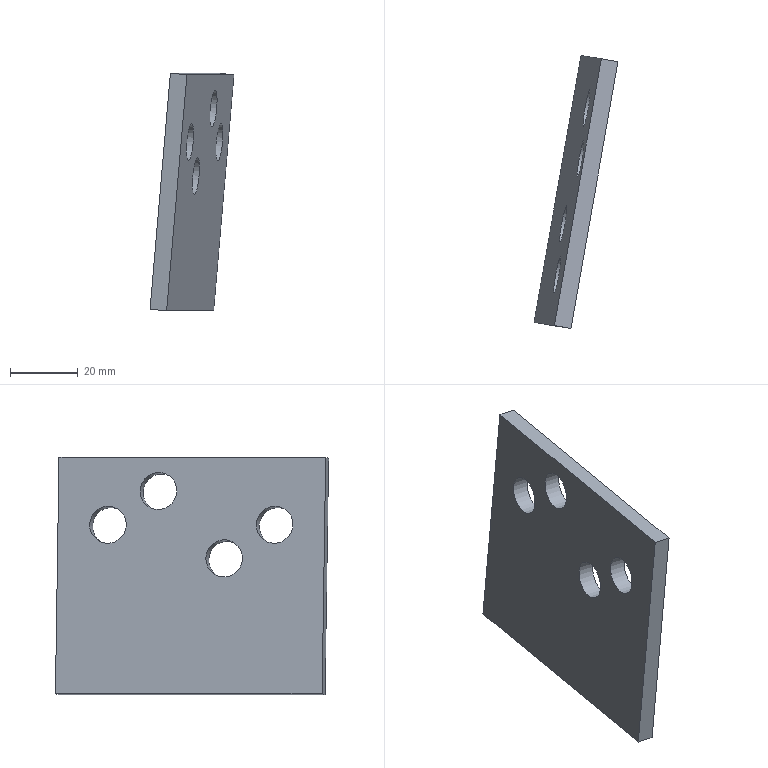Part | NX | features solid 2 | 1 solid | 10 faces | box 24.805 x 80.709 x 70.169 mm | volume 26099 mm3 | plane 6 | cylinder 4 | commonest cylinder face diameters 11 x4
STEP:
#1=CARTESIAN_POINT('',(390.845,64.104,71.411));
#2=VERTEX_POINT('',#1);
#3=CARTESIAN_POINT('',(376.953,-14.68,71.411));
#4=VERTEX_POINT('',#3);
#5=CARTESIAN_POINT('',(390.845,64.104,71.411));
#6=DIRECTION('',(0.1736,0.9848,0.));
#7=VECTOR('',#6,1000.);
#8=LINE('',#5,#7);
#9=EDGE_CURVE('',#2,#4,#8,.F.);
#10=ORIENTED_EDGE('',*,*,#9,.T.);
#11=CARTESIAN_POINT('',(381.858,-15.545,70.975));
#12=VERTEX_POINT('',#11);
#13=CARTESIAN_POINT('',(381.858,-15.545,70.975));
#14=DIRECTION('',(-0.9811,0.173,0.08716));
#15=VECTOR('',#14,1000.);
#16=LINE('',#13,#15);
#17=EDGE_CURVE('',#12,#4,#16,.T.);
#18=ORIENTED_EDGE('',*,*,#17,.F.);
#19=CARTESIAN_POINT('',(395.75,63.239,70.975));
#20=VERTEX_POINT('',#19);
#21=CARTESIAN_POINT('',(395.75,63.239,70.975));
#22=DIRECTION('',(0.1736,0.9848,0.));
#23=VECTOR('',#22,1000.);
#24=LINE('',#21,#23);
#25=EDGE_CURVE('',#20,#12,#24,.F.);
#26=ORIENTED_EDGE('',*,*,#25,.F.);
#27=CARTESIAN_POINT('',(395.75,63.239,70.975));
#28=DIRECTION('',(-0.9811,0.173,0.08716));
#29=VECTOR('',#28,1000.);
#30=LINE('',#27,#29);
#31=EDGE_CURVE('',#20,#2,#30,.T.);
#32=ORIENTED_EDGE('',*,*,#31,.T.);
#33=EDGE_LOOP('',(#10,#18,#26,#32));
#34=FACE_BOUND('',#33,.T.);
#35=CARTESIAN_POINT('',(395.75,63.239,70.975));
#36=DIRECTION('',(0.08583,-0.01513,0.9962));
#37=DIRECTION('',(-0.9963,0.,0.08584));
#38=AXIS2_PLACEMENT_3D('',#35,#36,#37);
#39=PLANE('',#38);
#40=ADVANCED_FACE('',(#34),#39,.T.);
#41=CARTESIAN_POINT('',(384.836,65.164,1.677));
#42=VERTEX_POINT('',#41);
#43=CARTESIAN_POINT('',(387.476,64.698,32.311));
#44=DIRECTION('',(-0.08583,0.01513,-0.9962));
#45=VECTOR('',#44,1000.);
#46=LINE('',#43,#45);
#47=EDGE_CURVE('',#2,#42,#46,.T.);
#48=ORIENTED_EDGE('',*,*,#47,.F.);
#49=ORIENTED_EDGE('',*,*,#31,.F.);
#50=CARTESIAN_POINT('',(389.742,64.299,1.241));
#51=VERTEX_POINT('',#50);
#52=CARTESIAN_POINT('',(392.381,63.833,31.876));
#53=DIRECTION('',(-0.08583,0.01513,-0.9962));
#54=VECTOR('',#53,1000.);
#55=LINE('',#52,#54);
#56=EDGE_CURVE('',#20,#51,#55,.T.);
#57=ORIENTED_EDGE('',*,*,#56,.T.);
#58=CARTESIAN_POINT('',(389.742,64.299,1.241));
#59=DIRECTION('',(0.9811,-0.173,-0.08716));
#60=VECTOR('',#59,1000.);
#61=LINE('',#58,#60);
#62=EDGE_CURVE('',#51,#42,#61,.F.);
#63=ORIENTED_EDGE('',*,*,#62,.T.);
#64=EDGE_LOOP('',(#48,#49,#57,#63));
#65=FACE_BOUND('',#64,.T.);
#66=CARTESIAN_POINT('',(392.381,63.833,31.876));
#67=DIRECTION('',(-0.1736,-0.9848,0.));
#68=DIRECTION('',(-0.9848,0.1736,0.));
#69=AXIS2_PLACEMENT_3D('',#66,#67,#68);
#70=PLANE('',#69);
#71=ADVANCED_FACE('',(#65),#70,.F.);
#72=CARTESIAN_POINT('',(375.85,-14.486,1.241));
#73=VERTEX_POINT('',#72);
#74=CARTESIAN_POINT('',(370.945,-13.621,1.677));
#75=VERTEX_POINT('',#74);
#76=CARTESIAN_POINT('',(375.85,-14.486,1.241));
#77=DIRECTION('',(0.9811,-0.173,-0.08716));
#78=VECTOR('',#77,1000.);
#79=LINE('',#76,#78);
#80=EDGE_CURVE('',#73,#75,#79,.F.);
#81=ORIENTED_EDGE('',*,*,#80,.T.);
#82=CARTESIAN_POINT('',(384.836,65.164,1.677));
#83=DIRECTION('',(0.1736,0.9848,0.));
#84=VECTOR('',#83,1000.);
#85=LINE('',#82,#84);
#86=EDGE_CURVE('',#75,#42,#85,.T.);
#87=ORIENTED_EDGE('',*,*,#86,.T.);
#88=ORIENTED_EDGE('',*,*,#62,.F.);
#89=CARTESIAN_POINT('',(389.742,64.299,1.241));
#90=DIRECTION('',(0.1736,0.9848,0.));
#91=VECTOR('',#90,1000.);
#92=LINE('',#89,#91);
#93=EDGE_CURVE('',#73,#51,#92,.T.);
#94=ORIENTED_EDGE('',*,*,#93,.F.);
#95=EDGE_LOOP('',(#81,#87,#88,#94));
#96=FACE_BOUND('',#95,.T.);
#97=CARTESIAN_POINT('',(389.742,64.299,1.241));
#98=DIRECTION('',(0.08583,-0.01513,0.9962));
#99=DIRECTION('',(-0.9963,0.,0.08584));
#100=AXIS2_PLACEMENT_3D('',#97,#98,#99);
#101=PLANE('',#100);
#102=ADVANCED_FACE('',(#96),#101,.F.);
#103=CARTESIAN_POINT('',(378.09,-14.881,84.61));
#104=DIRECTION('',(-0.08583,0.01513,-0.9962));
#105=VECTOR('',#104,1000.);
#106=LINE('',#103,#105);
#107=EDGE_CURVE('',#75,#4,#106,.F.);
#108=ORIENTED_EDGE('',*,*,#107,.F.);
#109=ORIENTED_EDGE('',*,*,#80,.F.);
#110=CARTESIAN_POINT('',(382.995,-15.746,84.174));
#111=DIRECTION('',(-0.08583,0.01513,-0.9962));
#112=VECTOR('',#111,1000.);
#113=LINE('',#110,#112);
#114=EDGE_CURVE('',#73,#12,#113,.F.);
#115=ORIENTED_EDGE('',*,*,#114,.T.);
#116=ORIENTED_EDGE('',*,*,#17,.T.);
#117=EDGE_LOOP('',(#108,#109,#115,#116));
#118=FACE_BOUND('',#117,.T.);
#119=CARTESIAN_POINT('',(382.995,-15.746,84.174));
#120=DIRECTION('',(0.1736,0.9848,0.));
#121=DIRECTION('',(0.9848,-0.1736,0.));
#122=AXIS2_PLACEMENT_3D('',#119,#120,#121);
#123=PLANE('',#122);
#124=ADVANCED_FACE('',(#118),#123,.F.);
#125=CARTESIAN_POINT('',(385.448,19.87,41.089));
#126=VERTEX_POINT('',#125);
#127=CARTESIAN_POINT('',(384.493,14.453,41.089));
#128=DIRECTION('',(0.9811,-0.173,-0.08716));
#129=DIRECTION('',(0.1736,0.9848,0.));
#130=AXIS2_PLACEMENT_3D('',#127,#128,#129);
#131=CIRCLE('',#130,5.5);
#132=EDGE_CURVE('',#126,#126,#131,.F.);
#133=ORIENTED_EDGE('',*,*,#132,.T.);
#134=EDGE_LOOP('',(#133));
#135=FACE_BOUND('',#134,.T.);
#136=CARTESIAN_POINT('',(390.637,39.263,61.013));
#137=VERTEX_POINT('',#136);
#138=CARTESIAN_POINT('',(389.682,33.847,61.013));
#139=DIRECTION('',(0.9811,-0.173,-0.08716));
#140=DIRECTION('',(0.1736,0.9848,0.));
#141=AXIS2_PLACEMENT_3D('',#138,#139,#140);
#142=CIRCLE('',#141,5.5);
#143=EDGE_CURVE('',#137,#137,#142,.F.);
#144=ORIENTED_EDGE('',*,*,#143,.T.);
#145=EDGE_LOOP('',(#144));
#146=FACE_BOUND('',#145,.T.);
#147=CARTESIAN_POINT('',(383.701,4.946,51.051));
#148=VERTEX_POINT('',#147);
#149=CARTESIAN_POINT('',(382.746,-0.4703,51.051));
#150=DIRECTION('',(0.9811,-0.173,-0.08716));
#151=DIRECTION('',(0.1736,0.9848,0.));
#152=AXIS2_PLACEMENT_3D('',#149,#150,#151);
#153=CIRCLE('',#152,5.5);
#154=EDGE_CURVE('',#148,#148,#153,.F.);
#155=ORIENTED_EDGE('',*,*,#154,.T.);
#156=EDGE_LOOP('',(#155));
#157=FACE_BOUND('',#156,.T.);
#158=CARTESIAN_POINT('',(392.384,54.187,51.051));
#159=VERTEX_POINT('',#158);
#160=CARTESIAN_POINT('',(391.429,48.77,51.051));
#161=DIRECTION('',(0.9811,-0.173,-0.08716));
#162=DIRECTION('',(0.1736,0.9848,0.));
#163=AXIS2_PLACEMENT_3D('',#160,#161,#162);
#164=CIRCLE('',#163,5.5);
#165=EDGE_CURVE('',#159,#159,#164,.F.);
#166=ORIENTED_EDGE('',*,*,#165,.T.);
#167=EDGE_LOOP('',(#166));
#168=FACE_BOUND('',#167,.T.);
#169=ORIENTED_EDGE('',*,*,#25,.T.);
#170=ORIENTED_EDGE('',*,*,#114,.F.);
#171=ORIENTED_EDGE('',*,*,#93,.T.);
#172=ORIENTED_EDGE('',*,*,#56,.F.);
#173=EDGE_LOOP('',(#169,#170,#171,#172));
#174=FACE_BOUND('',#173,.T.);
#175=CARTESIAN_POINT('',(396.887,63.039,84.174));
#176=DIRECTION('',(-0.9811,0.173,0.08716));
#177=DIRECTION('',(-0.1736,-0.9848,0.));
#178=AXIS2_PLACEMENT_3D('',#175,#176,#177);
#179=PLANE('',#178);
#180=ADVANCED_FACE('',(#135,#146,#157,#168,#174),#179,.F.);
#181=CARTESIAN_POINT('',(380.542,20.735,41.525));
#182=VERTEX_POINT('',#181);
#183=CARTESIAN_POINT('',(379.587,15.318,41.525));
#184=DIRECTION('',(0.9811,-0.173,-0.08716));
#185=DIRECTION('',(0.1736,0.9848,0.));
#186=AXIS2_PLACEMENT_3D('',#183,#184,#185);
#187=CIRCLE('',#186,5.5);
#188=EDGE_CURVE('',#182,#182,#187,.F.);
#189=ORIENTED_EDGE('',*,*,#188,.F.);
#190=EDGE_LOOP('',(#189));
#191=FACE_BOUND('',#190,.T.);
#192=CARTESIAN_POINT('',(385.732,40.128,61.449));
#193=VERTEX_POINT('',#192);
#194=CARTESIAN_POINT('',(384.777,34.712,61.449));
#195=DIRECTION('',(0.9811,-0.173,-0.08716));
#196=DIRECTION('',(0.1736,0.9848,0.));
#197=AXIS2_PLACEMENT_3D('',#194,#195,#196);
#198=CIRCLE('',#197,5.5);
#199=EDGE_CURVE('',#193,#193,#198,.F.);
#200=ORIENTED_EDGE('',*,*,#199,.F.);
#201=EDGE_LOOP('',(#200));
#202=FACE_BOUND('',#201,.T.);
#203=CARTESIAN_POINT('',(378.796,5.811,51.487));
#204=VERTEX_POINT('',#203);
#205=CARTESIAN_POINT('',(377.841,0.3946,51.487));
#206=DIRECTION('',(0.9811,-0.173,-0.08716));
#207=DIRECTION('',(0.1736,0.9848,0.));
#208=AXIS2_PLACEMENT_3D('',#205,#206,#207);
#209=CIRCLE('',#208,5.5);
#210=EDGE_CURVE('',#204,#204,#209,.F.);
#211=ORIENTED_EDGE('',*,*,#210,.F.);
#212=EDGE_LOOP('',(#211));
#213=FACE_BOUND('',#212,.T.);
#214=CARTESIAN_POINT('',(387.478,55.051,51.487));
#215=VERTEX_POINT('',#214);
#216=CARTESIAN_POINT('',(386.523,49.635,51.487));
#217=DIRECTION('',(0.9811,-0.173,-0.08716));
#218=DIRECTION('',(0.1736,0.9848,0.));
#219=AXIS2_PLACEMENT_3D('',#216,#217,#218);
#220=CIRCLE('',#219,5.5);
#221=EDGE_CURVE('',#215,#215,#220,.F.);
#222=ORIENTED_EDGE('',*,*,#221,.F.);
#223=EDGE_LOOP('',(#222));
#224=FACE_BOUND('',#223,.T.);
#225=ORIENTED_EDGE('',*,*,#9,.F.);
#226=ORIENTED_EDGE('',*,*,#47,.T.);
#227=ORIENTED_EDGE('',*,*,#86,.F.);
#228=ORIENTED_EDGE('',*,*,#107,.T.);
#229=EDGE_LOOP('',(#225,#226,#227,#228));
#230=FACE_BOUND('',#229,.T.);
#231=CARTESIAN_POINT('',(391.982,63.904,84.61));
#232=DIRECTION('',(-0.9811,0.173,0.08716));
#233=DIRECTION('',(-0.1736,-0.9848,0.));
#234=AXIS2_PLACEMENT_3D('',#231,#232,#233);
#235=PLANE('',#234);
#236=ADVANCED_FACE('',(#191,#202,#213,#224,#230),#235,.T.);
#237=ORIENTED_EDGE('',*,*,#165,.F.);
#238=EDGE_LOOP('',(#237));
#239=FACE_BOUND('',#238,.T.);
#240=ORIENTED_EDGE('',*,*,#221,.T.);
#241=EDGE_LOOP('',(#240));
#242=FACE_BOUND('',#241,.T.);
#243=CARTESIAN_POINT('',(293.323,66.069,59.767));
#244=DIRECTION('',(0.9811,-0.173,-0.08716));
#245=DIRECTION('',(-0.1736,-0.9848,0.));
#246=AXIS2_PLACEMENT_3D('',#243,#244,#245);
#247=CYLINDRICAL_SURFACE('',#246,5.5);
#248=ADVANCED_FACE('',(#239,#242),#247,.F.);
#249=ORIENTED_EDGE('',*,*,#154,.F.);
#250=EDGE_LOOP('',(#249));
#251=FACE_BOUND('',#250,.T.);
#252=ORIENTED_EDGE('',*,*,#210,.T.);
#253=EDGE_LOOP('',(#252));
#254=FACE_BOUND('',#253,.T.);
#255=CARTESIAN_POINT('',(284.64,16.828,59.767));
#256=DIRECTION('',(0.9811,-0.173,-0.08716));
#257=DIRECTION('',(-0.1736,-0.9848,0.));
#258=AXIS2_PLACEMENT_3D('',#255,#256,#257);
#259=CYLINDRICAL_SURFACE('',#258,5.5);
#260=ADVANCED_FACE('',(#251,#254),#259,.F.);
#261=ORIENTED_EDGE('',*,*,#143,.F.);
#262=EDGE_LOOP('',(#261));
#263=FACE_BOUND('',#262,.T.);
#264=ORIENTED_EDGE('',*,*,#199,.T.);
#265=EDGE_LOOP('',(#264));
#266=FACE_BOUND('',#265,.T.);
#267=CARTESIAN_POINT('',(291.576,51.145,69.729));
#268=DIRECTION('',(0.9811,-0.173,-0.08716));
#269=DIRECTION('',(-0.1736,-0.9848,0.));
#270=AXIS2_PLACEMENT_3D('',#267,#268,#269);
#271=CYLINDRICAL_SURFACE('',#270,5.5);
#272=ADVANCED_FACE('',(#263,#266),#271,.F.);
#273=ORIENTED_EDGE('',*,*,#132,.F.);
#274=EDGE_LOOP('',(#273));
#275=FACE_BOUND('',#274,.T.);
#276=ORIENTED_EDGE('',*,*,#188,.T.);
#277=EDGE_LOOP('',(#276));
#278=FACE_BOUND('',#277,.T.);
#279=CARTESIAN_POINT('',(315.818,26.562,47.19));
#280=DIRECTION('',(0.9811,-0.173,-0.08716));
#281=DIRECTION('',(-0.1736,-0.9848,0.));
#282=AXIS2_PLACEMENT_3D('',#279,#280,#281);
#283=CYLINDRICAL_SURFACE('',#282,5.5);
#284=ADVANCED_FACE('',(#275,#278),#283,.F.);
#285=CLOSED_SHELL('',(#40,#71,#102,#124,#180,#236,#248,#260,#272,#284));
#286=MANIFOLD_SOLID_BREP('',#285);
#287=(LENGTH_UNIT()NAMED_UNIT(*)SI_UNIT(.MILLI.,.METRE.));
#288=UNCERTAINTY_MEASURE_WITH_UNIT(LENGTH_MEASURE(0.00001),#287,'','');
#289=(NAMED_UNIT(*)PLANE_ANGLE_UNIT()SI_UNIT($,.RADIAN.));
#290=(NAMED_UNIT(*)SI_UNIT($,.STERADIAN.)SOLID_ANGLE_UNIT());
#291=(GEOMETRIC_REPRESENTATION_CONTEXT(3)GLOBAL_UNCERTAINTY_ASSIGNED_CONTEXT((#288))GLOBAL_UNIT_ASSIGNED_CONTEXT((#287,#289,#290))REPRESENTATION_CONTEXT('',''));
#292=ADVANCED_BREP_SHAPE_REPRESENTATION('',(#286),#291);